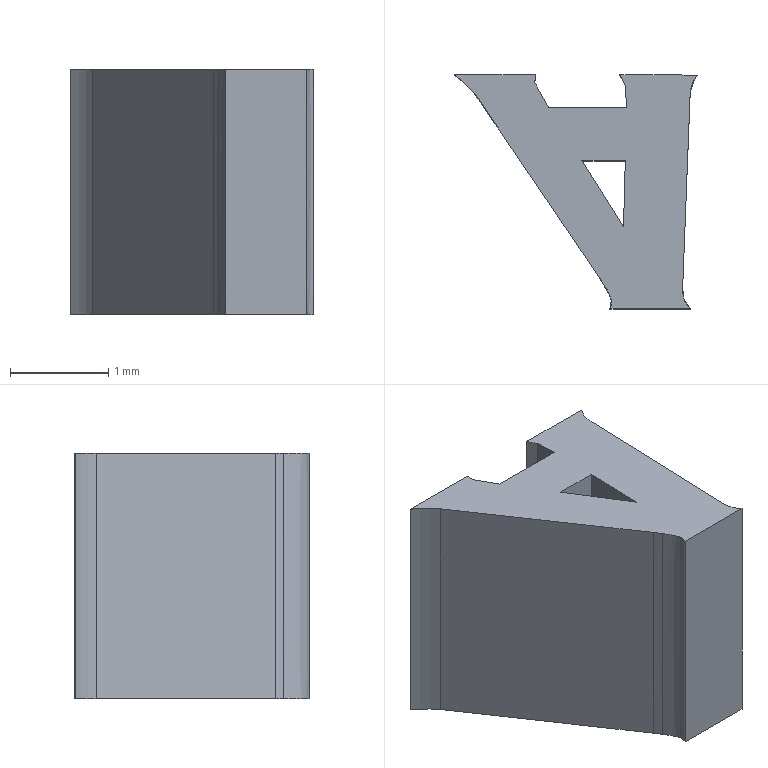Part | STEP file | lll_id1098_x_t | 1 solid | 20 faces | box 2.479 x 2.385 x 2.5 mm | volume 7.725 mm3 | plane 14 | other 4 | cylinder 2 | commonest cylinder face diameters 1.645 x1 55.723 x1
STEP:
#1=CARTESIAN_POINT('',(387.646,-127.04,2.35));
#2=VERTEX_POINT('',#1);
#3=CARTESIAN_POINT('',(387.664,-126.366,2.35));
#4=VERTEX_POINT('',#3);
#5=CARTESIAN_POINT('',(387.646,-127.04,2.35));
#6=DIRECTION('',(0.02693,0.9996,0.));
#7=VECTOR('',#6,1.);
#8=LINE('',#5,#7);
#9=EDGE_CURVE('',#2,#4,#8,.T.);
#10=ORIENTED_EDGE('',*,*,#9,.T.);
#11=CARTESIAN_POINT('',(387.664,-126.366,-0.15));
#12=VERTEX_POINT('',#11);
#13=CARTESIAN_POINT('',(387.664,-126.366,-0.15));
#14=DIRECTION('',(0.,0.,1.));
#15=VECTOR('',#14,1.);
#16=LINE('',#13,#15);
#17=EDGE_CURVE('',#12,#4,#16,.T.);
#18=ORIENTED_EDGE('',*,*,#17,.F.);
#19=CARTESIAN_POINT('',(387.646,-127.04,-0.15));
#20=VERTEX_POINT('',#19);
#21=CARTESIAN_POINT('',(387.646,-127.04,-0.15));
#22=DIRECTION('',(0.02693,0.9996,0.));
#23=VECTOR('',#22,1.);
#24=LINE('',#21,#23);
#25=EDGE_CURVE('',#20,#12,#24,.T.);
#26=ORIENTED_EDGE('',*,*,#25,.F.);
#27=CARTESIAN_POINT('',(387.646,-127.04,-0.15));
#28=DIRECTION('',(0.,0.,1.));
#29=VECTOR('',#28,1.);
#30=LINE('',#27,#29);
#31=EDGE_CURVE('',#20,#2,#30,.T.);
#32=ORIENTED_EDGE('',*,*,#31,.T.);
#33=EDGE_LOOP('',(#10,#18,#26,#32));
#34=FACE_OUTER_BOUND('',#33,.T.);
#35=CARTESIAN_POINT('',(387.646,-127.04,-0.15));
#36=DIRECTION('',(0.9996,-0.02693,0.));
#37=DIRECTION('',(-0.02693,-0.9996,0.));
#38=AXIS2_PLACEMENT_3D('',#35,#36,#37);
#39=PLANE('',#38);
#40=ADVANCED_FACE('',(#34),#39,.F.);
#41=CARTESIAN_POINT('',(387.223,-126.366,2.35));
#42=VERTEX_POINT('',#41);
#43=CARTESIAN_POINT('',(387.664,-126.366,2.35));
#44=DIRECTION('',(-1.,0.,0.));
#45=VECTOR('',#44,1.);
#46=LINE('',#43,#45);
#47=EDGE_CURVE('',#4,#42,#46,.T.);
#48=ORIENTED_EDGE('',*,*,#47,.T.);
#49=CARTESIAN_POINT('',(387.223,-126.366,-0.15));
#50=VERTEX_POINT('',#49);
#51=CARTESIAN_POINT('',(387.223,-126.366,-0.15));
#52=DIRECTION('',(0.,0.,1.));
#53=VECTOR('',#52,1.);
#54=LINE('',#51,#53);
#55=EDGE_CURVE('',#50,#42,#54,.T.);
#56=ORIENTED_EDGE('',*,*,#55,.F.);
#57=CARTESIAN_POINT('',(387.664,-126.366,-0.15));
#58=DIRECTION('',(-1.,0.,0.));
#59=VECTOR('',#58,1.);
#60=LINE('',#57,#59);
#61=EDGE_CURVE('',#12,#50,#60,.T.);
#62=ORIENTED_EDGE('',*,*,#61,.F.);
#63=ORIENTED_EDGE('',*,*,#17,.T.);
#64=EDGE_LOOP('',(#48,#56,#62,#63));
#65=FACE_OUTER_BOUND('',#64,.T.);
#66=CARTESIAN_POINT('',(387.664,-126.366,-0.15));
#67=DIRECTION('',(0.,1.,0.));
#68=DIRECTION('',(0.,0.,1.));
#69=AXIS2_PLACEMENT_3D('',#66,#67,#68);
#70=PLANE('',#69);
#71=ADVANCED_FACE('',(#65),#70,.F.);
#72=CARTESIAN_POINT('',(388.398,-125.498,2.35));
#73=VERTEX_POINT('',#72);
#74=CARTESIAN_POINT('',(388.323,-125.704,2.35));
#75=VERTEX_POINT('',#74);
#76=CARTESIAN_POINT('',(388.398,-125.498,2.35));
#77=CARTESIAN_POINT('',(388.389,-125.508,2.35));
#78=CARTESIAN_POINT('',(388.38,-125.519,2.35));
#79=CARTESIAN_POINT('',(388.363,-125.544,2.35));
#80=CARTESIAN_POINT('',(388.355,-125.559,2.35));
#81=CARTESIAN_POINT('',(388.343,-125.589,2.35));
#82=CARTESIAN_POINT('',(388.338,-125.605,2.35));
#83=CARTESIAN_POINT('',(388.331,-125.632,2.35));
#84=CARTESIAN_POINT('',(388.329,-125.644,2.35));
#85=CARTESIAN_POINT('',(388.325,-125.672,2.35));
#86=CARTESIAN_POINT('',(388.324,-125.688,2.35));
#87=CARTESIAN_POINT('',(388.323,-125.704,2.35));
#88=(BOUNDED_CURVE()B_SPLINE_CURVE(3,(#76,#77,#78,#79,#80,#81,#82,#83,#84,#85,#86,#87),.UNSPECIFIED.,.F.,.F.)B_SPLINE_CURVE_WITH_KNOTS((4,2,2,2,2,4),(0.,0.1892,0.4077,0.6263,0.7817,1.),.UNSPECIFIED.)CURVE()GEOMETRIC_REPRESENTATION_ITEM()RATIONAL_B_SPLINE_CURVE((0.5006,0.4998,0.4998,0.499,0.499,0.4995,0.4995,0.5003,0.5003,0.5002,0.5002,0.5006))REPRESENTATION_ITEM(''));
#89=EDGE_CURVE('',#73,#75,#88,.T.);
#90=ORIENTED_EDGE('',*,*,#89,.T.);
#91=CARTESIAN_POINT('',(388.323,-125.704,-0.15));
#92=VERTEX_POINT('',#91);
#93=CARTESIAN_POINT('',(388.323,-125.704,-0.15));
#94=DIRECTION('',(0.,0.,1.));
#95=VECTOR('',#94,1.);
#96=LINE('',#93,#95);
#97=EDGE_CURVE('',#92,#75,#96,.T.);
#98=ORIENTED_EDGE('',*,*,#97,.F.);
#99=CARTESIAN_POINT('',(388.398,-125.498,-0.15));
#100=VERTEX_POINT('',#99);
#101=CARTESIAN_POINT('',(388.398,-125.498,-0.15));
#102=CARTESIAN_POINT('',(388.389,-125.508,-0.15));
#103=CARTESIAN_POINT('',(388.38,-125.519,-0.15));
#104=CARTESIAN_POINT('',(388.363,-125.544,-0.15));
#105=CARTESIAN_POINT('',(388.355,-125.559,-0.15));
#106=CARTESIAN_POINT('',(388.343,-125.589,-0.15));
#107=CARTESIAN_POINT('',(388.338,-125.605,-0.15));
#108=CARTESIAN_POINT('',(388.331,-125.632,-0.15));
#109=CARTESIAN_POINT('',(388.329,-125.644,-0.15));
#110=CARTESIAN_POINT('',(388.325,-125.672,-0.15));
#111=CARTESIAN_POINT('',(388.324,-125.688,-0.15));
#112=CARTESIAN_POINT('',(388.323,-125.704,-0.15));
#113=(BOUNDED_CURVE()B_SPLINE_CURVE(3,(#101,#102,#103,#104,#105,#106,#107,#108,#109,#110,#111,#112),.UNSPECIFIED.,.F.,.F.)B_SPLINE_CURVE_WITH_KNOTS((4,2,2,2,2,4),(0.,0.1892,0.4077,0.6263,0.7817,1.),.UNSPECIFIED.)CURVE()GEOMETRIC_REPRESENTATION_ITEM()RATIONAL_B_SPLINE_CURVE((0.5006,0.4998,0.4998,0.499,0.499,0.4995,0.4995,0.5003,0.5003,0.5002,0.5002,0.5006))REPRESENTATION_ITEM(''));
#114=EDGE_CURVE('',#100,#92,#113,.T.);
#115=ORIENTED_EDGE('',*,*,#114,.F.);
#116=CARTESIAN_POINT('',(388.398,-125.498,-0.15));
#117=DIRECTION('',(0.,0.,1.));
#118=VECTOR('',#117,1.);
#119=LINE('',#116,#118);
#120=EDGE_CURVE('',#100,#73,#119,.T.);
#121=ORIENTED_EDGE('',*,*,#120,.T.);
#122=EDGE_LOOP('',(#90,#98,#115,#121));
#123=FACE_OUTER_BOUND('',#122,.T.);
#124=CARTESIAN_POINT('',(388.398,-125.498,-0.15));
#125=CARTESIAN_POINT('',(388.389,-125.508,-0.15));
#126=CARTESIAN_POINT('',(388.38,-125.519,-0.15));
#127=CARTESIAN_POINT('',(388.363,-125.544,-0.15));
#128=CARTESIAN_POINT('',(388.355,-125.559,-0.15));
#129=CARTESIAN_POINT('',(388.343,-125.589,-0.15));
#130=CARTESIAN_POINT('',(388.338,-125.605,-0.15));
#131=CARTESIAN_POINT('',(388.331,-125.632,-0.15));
#132=CARTESIAN_POINT('',(388.329,-125.644,-0.15));
#133=CARTESIAN_POINT('',(388.325,-125.672,-0.15));
#134=CARTESIAN_POINT('',(388.324,-125.688,-0.15));
#135=CARTESIAN_POINT('',(388.323,-125.704,-0.15));
#136=(BOUNDED_CURVE()B_SPLINE_CURVE(3,(#124,#125,#126,#127,#128,#129,#130,#131,#132,#133,#134,#135),.UNSPECIFIED.,.F.,.F.)B_SPLINE_CURVE_WITH_KNOTS((4,2,2,2,2,4),(0.,0.1892,0.4077,0.6263,0.7817,1.),.UNSPECIFIED.)CURVE()GEOMETRIC_REPRESENTATION_ITEM()RATIONAL_B_SPLINE_CURVE((0.5006,0.4998,0.4998,0.499,0.499,0.4995,0.4995,0.5003,0.5003,0.5002,0.5002,0.5006))REPRESENTATION_ITEM(''));
#137=DIRECTION('',(0.,0.,1.));
#138=VECTOR('',#137,1.);
#139=SURFACE_OF_LINEAR_EXTRUSION('',#136,#138);
#140=ADVANCED_FACE('',(#123),#139,.F.);
#141=CARTESIAN_POINT('',(388.247,-127.665,2.35));
#142=VERTEX_POINT('',#141);
#143=CARTESIAN_POINT('',(388.323,-125.704,2.35));
#144=DIRECTION('',(-0.0386,-0.9993,0.));
#145=VECTOR('',#144,1.);
#146=LINE('',#143,#145);
#147=EDGE_CURVE('',#75,#142,#146,.T.);
#148=ORIENTED_EDGE('',*,*,#147,.T.);
#149=CARTESIAN_POINT('',(388.247,-127.665,-0.15));
#150=VERTEX_POINT('',#149);
#151=CARTESIAN_POINT('',(388.247,-127.665,-0.15));
#152=DIRECTION('',(0.,0.,1.));
#153=VECTOR('',#152,1.);
#154=LINE('',#151,#153);
#155=EDGE_CURVE('',#150,#142,#154,.T.);
#156=ORIENTED_EDGE('',*,*,#155,.F.);
#157=CARTESIAN_POINT('',(388.323,-125.704,-0.15));
#158=DIRECTION('',(-0.0386,-0.9993,0.));
#159=VECTOR('',#158,1.);
#160=LINE('',#157,#159);
#161=EDGE_CURVE('',#92,#150,#160,.T.);
#162=ORIENTED_EDGE('',*,*,#161,.F.);
#163=ORIENTED_EDGE('',*,*,#97,.T.);
#164=EDGE_LOOP('',(#148,#156,#162,#163));
#165=FACE_OUTER_BOUND('',#164,.T.);
#166=CARTESIAN_POINT('',(388.323,-125.704,-0.15));
#167=DIRECTION('',(-0.9993,0.0386,0.));
#168=DIRECTION('',(0.0386,0.9993,0.));
#169=AXIS2_PLACEMENT_3D('',#166,#167,#168);
#170=PLANE('',#169);
#171=ADVANCED_FACE('',(#165),#170,.F.);
#172=CARTESIAN_POINT('',(388.323,-127.874,2.35));
#173=VERTEX_POINT('',#172);
#174=CARTESIAN_POINT('',(388.247,-127.665,2.35));
#175=CARTESIAN_POINT('',(388.246,-127.686,2.35));
#176=CARTESIAN_POINT('',(388.248,-127.708,2.35));
#177=CARTESIAN_POINT('',(388.253,-127.746,2.35));
#178=CARTESIAN_POINT('',(388.257,-127.762,2.35));
#179=CARTESIAN_POINT('',(388.271,-127.802,2.35));
#180=CARTESIAN_POINT('',(388.283,-127.825,2.35));
#181=CARTESIAN_POINT('',(388.307,-127.855,2.35));
#182=CARTESIAN_POINT('',(388.315,-127.864,2.35));
#183=CARTESIAN_POINT('',(388.324,-127.872,2.35));
#184=(BOUNDED_CURVE()B_SPLINE_CURVE(3,(#174,#175,#176,#177,#178,#179,#180,#181,#182,#183),.UNSPECIFIED.,.F.,.F.)B_SPLINE_CURVE_WITH_KNOTS((4,2,2,2,4),(0.,0.2836,0.5035,0.8455,1.),.UNSPECIFIED.)CURVE()GEOMETRIC_REPRESENTATION_ITEM()RATIONAL_B_SPLINE_CURVE((0.5011,0.4996,0.4996,0.4997,0.4997,0.4954,0.4954,0.5003,0.5003,0.5011))REPRESENTATION_ITEM(''));
#185=EDGE_CURVE('',#142,#173,#184,.T.);
#186=ORIENTED_EDGE('',*,*,#185,.T.);
#187=CARTESIAN_POINT('',(388.323,-127.874,-0.15));
#188=VERTEX_POINT('',#187);
#189=CARTESIAN_POINT('',(388.329,-127.876,-0.15));
#190=DIRECTION('',(0.,0.,1.));
#191=VECTOR('',#190,1.);
#192=LINE('',#189,#191);
#193=EDGE_CURVE('',#188,#173,#192,.T.);
#194=ORIENTED_EDGE('',*,*,#193,.F.);
#195=CARTESIAN_POINT('',(388.247,-127.665,-0.15));
#196=CARTESIAN_POINT('',(388.246,-127.686,-0.15));
#197=CARTESIAN_POINT('',(388.248,-127.708,-0.15));
#198=CARTESIAN_POINT('',(388.253,-127.746,-0.15));
#199=CARTESIAN_POINT('',(388.257,-127.762,-0.15));
#200=CARTESIAN_POINT('',(388.271,-127.802,-0.15));
#201=CARTESIAN_POINT('',(388.283,-127.825,-0.15));
#202=CARTESIAN_POINT('',(388.307,-127.855,-0.15));
#203=CARTESIAN_POINT('',(388.315,-127.864,-0.15));
#204=CARTESIAN_POINT('',(388.325,-127.872,-0.15));
#205=CARTESIAN_POINT('',(388.325,-127.873,-0.15));
#206=CARTESIAN_POINT('',(388.326,-127.873,-0.15));
#207=(BOUNDED_CURVE()B_SPLINE_CURVE(3,(#195,#196,#197,#198,#199,#200,#201,#202,#203,#204,#205,#206),.UNSPECIFIED.,.F.,.F.)B_SPLINE_CURVE_WITH_KNOTS((4,2,2,2,2,4),(0.,0.2808,0.4985,0.8371,0.9901,1.),.UNSPECIFIED.)CURVE()GEOMETRIC_REPRESENTATION_ITEM()RATIONAL_B_SPLINE_CURVE((0.5011,0.4996,0.4996,0.4997,0.4997,0.4954,0.4954,0.5003,0.5003,0.5011,0.5011,0.5011))REPRESENTATION_ITEM(''));
#208=EDGE_CURVE('',#150,#188,#207,.T.);
#209=ORIENTED_EDGE('',*,*,#208,.F.);
#210=ORIENTED_EDGE('',*,*,#155,.T.);
#211=EDGE_LOOP('',(#186,#194,#209,#210));
#212=FACE_OUTER_BOUND('',#211,.T.);
#213=CARTESIAN_POINT('',(388.247,-127.665,-0.15));
#214=CARTESIAN_POINT('',(388.246,-127.686,-0.15));
#215=CARTESIAN_POINT('',(388.248,-127.708,-0.15));
#216=CARTESIAN_POINT('',(388.253,-127.746,-0.15));
#217=CARTESIAN_POINT('',(388.257,-127.762,-0.15));
#218=CARTESIAN_POINT('',(388.271,-127.802,-0.15));
#219=CARTESIAN_POINT('',(388.283,-127.825,-0.15));
#220=CARTESIAN_POINT('',(388.307,-127.855,-0.15));
#221=CARTESIAN_POINT('',(388.315,-127.864,-0.15));
#222=CARTESIAN_POINT('',(388.325,-127.872,-0.15));
#223=CARTESIAN_POINT('',(388.325,-127.873,-0.15));
#224=CARTESIAN_POINT('',(388.326,-127.874,-0.15));
#225=CARTESIAN_POINT('',(388.327,-127.874,-0.15));
#226=CARTESIAN_POINT('',(388.328,-127.875,-0.15));
#227=CARTESIAN_POINT('',(388.328,-127.876,-0.15));
#228=CARTESIAN_POINT('',(388.329,-127.876,-0.15));
#229=(BOUNDED_CURVE()B_SPLINE_CURVE(3,(#213,#214,#215,#216,#217,#218,#219,#220,#221,#222,#223,#224,#225,#226,#227,#228),.UNSPECIFIED.,.F.,.F.)B_SPLINE_CURVE_WITH_KNOTS((4,2,2,2,2,2,2,4),(0.,0.2753,0.4887,0.8206,0.9706,0.9803,0.9901,1.),.UNSPECIFIED.)CURVE()GEOMETRIC_REPRESENTATION_ITEM()RATIONAL_B_SPLINE_CURVE((0.5011,0.4996,0.4996,0.4997,0.4997,0.4954,0.4954,0.5003,0.5003,0.5011,0.5011,0.5011,0.5011,0.5011,0.5011,0.5011))REPRESENTATION_ITEM(''));
#230=DIRECTION('',(0.,0.,1.));
#231=VECTOR('',#230,1.);
#232=SURFACE_OF_LINEAR_EXTRUSION('',#229,#231);
#233=ADVANCED_FACE('',(#212),#232,.F.);
#234=CARTESIAN_POINT('',(387.509,-127.874,2.35));
#235=VERTEX_POINT('',#234);
#236=CARTESIAN_POINT('',(388.323,-127.876,2.35));
#237=DIRECTION('',(-1.,0.,0.));
#238=VECTOR('',#237,1.);
#239=LINE('',#236,#238);
#240=EDGE_CURVE('',#173,#235,#239,.T.);
#241=ORIENTED_EDGE('',*,*,#240,.T.);
#242=CARTESIAN_POINT('',(387.509,-127.874,-0.15));
#243=VERTEX_POINT('',#242);
#244=CARTESIAN_POINT('',(387.507,-127.876,-0.15));
#245=DIRECTION('',(0.,0.,1.));
#246=VECTOR('',#245,1.);
#247=LINE('',#244,#246);
#248=EDGE_CURVE('',#243,#235,#247,.T.);
#249=ORIENTED_EDGE('',*,*,#248,.F.);
#250=CARTESIAN_POINT('',(388.323,-127.876,-0.15));
#251=DIRECTION('',(-1.,0.,0.));
#252=VECTOR('',#251,1.);
#253=LINE('',#250,#252);
#254=EDGE_CURVE('',#188,#243,#253,.T.);
#255=ORIENTED_EDGE('',*,*,#254,.F.);
#256=ORIENTED_EDGE('',*,*,#193,.T.);
#257=EDGE_LOOP('',(#241,#249,#255,#256));
#258=FACE_OUTER_BOUND('',#257,.T.);
#259=CARTESIAN_POINT('',(388.323,-127.876,-0.15));
#260=DIRECTION('',(0.,1.,0.));
#261=DIRECTION('',(0.,0.,1.));
#262=AXIS2_PLACEMENT_3D('',#259,#260,#261);
#263=PLANE('',#262);
#264=ADVANCED_FACE('',(#258),#263,.F.);
#265=CARTESIAN_POINT('',(387.437,-127.612,2.35));
#266=VERTEX_POINT('',#265);
#267=CARTESIAN_POINT('',(387.509,-127.872,2.35));
#268=CARTESIAN_POINT('',(387.511,-127.867,2.35));
#269=CARTESIAN_POINT('',(387.513,-127.861,2.35));
#270=CARTESIAN_POINT('',(387.523,-127.833,2.35));
#271=CARTESIAN_POINT('',(387.524,-127.809,2.35));
#272=CARTESIAN_POINT('',(387.518,-127.772,2.35));
#273=CARTESIAN_POINT('',(387.515,-127.759,2.35));
#274=CARTESIAN_POINT('',(387.507,-127.739,2.35));
#275=CARTESIAN_POINT('',(387.504,-127.731,2.35));
#276=CARTESIAN_POINT('',(387.496,-127.714,2.35));
#277=CARTESIAN_POINT('',(387.491,-127.703,2.35));
#278=CARTESIAN_POINT('',(387.48,-127.683,2.35));
#279=CARTESIAN_POINT('',(387.474,-127.672,2.35));
#280=CARTESIAN_POINT('',(387.458,-127.646,2.35));
#281=CARTESIAN_POINT('',(387.447,-127.629,2.35));
#282=CARTESIAN_POINT('',(387.437,-127.612,2.35));
#283=(BOUNDED_CURVE()B_SPLINE_CURVE(3,(#267,#268,#269,#270,#271,#272,#273,#274,#275,#276,#277,#278,#279,#280,#281,#282),.UNSPECIFIED.,.F.,.F.)B_SPLINE_CURVE_WITH_KNOTS((4,2,2,2,2,2,2,4),(0.,0.06399,0.3162,0.4617,0.5445,0.6686,0.7929,1.),.UNSPECIFIED.)CURVE()GEOMETRIC_REPRESENTATION_ITEM()RATIONAL_B_SPLINE_CURVE((0.5002,0.4999,0.4999,0.4907,0.4907,0.4986,0.4986,0.5,0.5,0.5,0.5,0.5002,0.5002,0.5002,0.5002,0.5002))REPRESENTATION_ITEM(''));
#284=EDGE_CURVE('',#235,#266,#283,.T.);
#285=ORIENTED_EDGE('',*,*,#284,.T.);
#286=CARTESIAN_POINT('',(387.437,-127.612,-0.15));
#287=VERTEX_POINT('',#286);
#288=CARTESIAN_POINT('',(387.437,-127.612,-0.15));
#289=DIRECTION('',(0.,0.,1.));
#290=VECTOR('',#289,1.);
#291=LINE('',#288,#290);
#292=EDGE_CURVE('',#287,#266,#291,.T.);
#293=ORIENTED_EDGE('',*,*,#292,.F.);
#294=CARTESIAN_POINT('',(387.507,-127.874,-0.15));
#295=CARTESIAN_POINT('',(387.508,-127.874,-0.15));
#296=CARTESIAN_POINT('',(387.508,-127.873,-0.15));
#297=CARTESIAN_POINT('',(387.511,-127.867,-0.15));
#298=CARTESIAN_POINT('',(387.513,-127.861,-0.15));
#299=CARTESIAN_POINT('',(387.523,-127.833,-0.15));
#300=CARTESIAN_POINT('',(387.524,-127.809,-0.15));
#301=CARTESIAN_POINT('',(387.518,-127.772,-0.15));
#302=CARTESIAN_POINT('',(387.515,-127.759,-0.15));
#303=CARTESIAN_POINT('',(387.507,-127.739,-0.15));
#304=CARTESIAN_POINT('',(387.504,-127.731,-0.15));
#305=CARTESIAN_POINT('',(387.496,-127.714,-0.15));
#306=CARTESIAN_POINT('',(387.491,-127.703,-0.15));
#307=CARTESIAN_POINT('',(387.48,-127.683,-0.15));
#308=CARTESIAN_POINT('',(387.474,-127.672,-0.15));
#309=CARTESIAN_POINT('',(387.458,-127.646,-0.15));
#310=CARTESIAN_POINT('',(387.447,-127.629,-0.15));
#311=CARTESIAN_POINT('',(387.437,-127.612,-0.15));
#312=(BOUNDED_CURVE()B_SPLINE_CURVE(3,(#294,#295,#296,#297,#298,#299,#300,#301,#302,#303,#304,#305,#306,#307,#308,#309,#310,#311),.UNSPECIFIED.,.F.,.F.)B_SPLINE_CURVE_WITH_KNOTS((4,2,2,2,2,2,2,2,4),(0.,0.009901,0.07326,0.323,0.467,0.549,0.6718,0.795,1.),.UNSPECIFIED.)CURVE()GEOMETRIC_REPRESENTATION_ITEM()RATIONAL_B_SPLINE_CURVE((0.5002,0.5002,0.5002,0.4999,0.4999,0.4907,0.4907,0.4986,0.4986,0.5,0.5,0.5,0.5,0.5002,0.5002,0.5002,0.5002,0.5002))REPRESENTATION_ITEM(''));
#313=EDGE_CURVE('',#243,#287,#312,.T.);
#314=ORIENTED_EDGE('',*,*,#313,.F.);
#315=ORIENTED_EDGE('',*,*,#248,.T.);
#316=EDGE_LOOP('',(#285,#293,#314,#315));
#317=FACE_OUTER_BOUND('',#316,.T.);
#318=CARTESIAN_POINT('',(387.506,-127.877,-0.15));
#319=CARTESIAN_POINT('',(387.507,-127.876,-0.15));
#320=CARTESIAN_POINT('',(387.507,-127.875,-0.15));
#321=CARTESIAN_POINT('',(387.508,-127.874,-0.15));
#322=CARTESIAN_POINT('',(387.508,-127.873,-0.15));
#323=CARTESIAN_POINT('',(387.511,-127.867,-0.15));
#324=CARTESIAN_POINT('',(387.513,-127.861,-0.15));
#325=CARTESIAN_POINT('',(387.523,-127.833,-0.15));
#326=CARTESIAN_POINT('',(387.524,-127.809,-0.15));
#327=CARTESIAN_POINT('',(387.518,-127.772,-0.15));
#328=CARTESIAN_POINT('',(387.515,-127.759,-0.15));
#329=CARTESIAN_POINT('',(387.507,-127.739,-0.15));
#330=CARTESIAN_POINT('',(387.504,-127.731,-0.15));
#331=CARTESIAN_POINT('',(387.496,-127.714,-0.15));
#332=CARTESIAN_POINT('',(387.491,-127.703,-0.15));
#333=CARTESIAN_POINT('',(387.48,-127.683,-0.15));
#334=CARTESIAN_POINT('',(387.474,-127.672,-0.15));
#335=CARTESIAN_POINT('',(387.458,-127.646,-0.15));
#336=CARTESIAN_POINT('',(387.447,-127.629,-0.15));
#337=CARTESIAN_POINT('',(387.437,-127.612,-0.15));
#338=(BOUNDED_CURVE()B_SPLINE_CURVE(3,(#318,#319,#320,#321,#322,#323,#324,#325,#326,#327,#328,#329,#330,#331,#332,#333,#334,#335,#336,#337),.UNSPECIFIED.,.F.,.F.)B_SPLINE_CURVE_WITH_KNOTS((4,2,2,2,2,2,2,2,2,4),(0.,0.009901,0.0197,0.08244,0.3297,0.4723,0.5535,0.6751,0.797,1.),.UNSPECIFIED.)CURVE()GEOMETRIC_REPRESENTATION_ITEM()RATIONAL_B_SPLINE_CURVE((0.5002,0.5002,0.5002,0.5002,0.5002,0.4999,0.4999,0.4907,0.4907,0.4986,0.4986,0.5,0.5,0.5,0.5,0.5002,0.5002,0.5002,0.5002,0.5002))REPRESENTATION_ITEM(''));
#339=DIRECTION('',(0.,0.,1.));
#340=VECTOR('',#339,1.);
#341=SURFACE_OF_LINEAR_EXTRUSION('',#338,#340);
#342=ADVANCED_FACE('',(#317),#341,.F.);
#343=CARTESIAN_POINT('',(387.387,-127.533,2.35));
#344=VERTEX_POINT('',#343);
#345=CARTESIAN_POINT('',(387.437,-127.612,2.35));
#346=CARTESIAN_POINT('',(387.429,-127.599,2.35));
#347=CARTESIAN_POINT('',(387.421,-127.585,2.35));
#348=CARTESIAN_POINT('',(387.404,-127.559,2.35));
#349=CARTESIAN_POINT('',(387.396,-127.546,2.35));
#350=CARTESIAN_POINT('',(387.387,-127.533,2.35));
#351=(BOUNDED_CURVE()B_SPLINE_CURVE(3,(#345,#346,#347,#348,#349,#350),.UNSPECIFIED.,.F.,.F.)B_SPLINE_CURVE_WITH_KNOTS((4,2,4),(0.,0.5001,1.),.UNSPECIFIED.)CURVE()GEOMETRIC_REPRESENTATION_ITEM()RATIONAL_B_SPLINE_CURVE((0.5002,0.5002,0.5002,0.5002,0.5002,0.5002))REPRESENTATION_ITEM(''));
#352=EDGE_CURVE('',#266,#344,#351,.T.);
#353=ORIENTED_EDGE('',*,*,#352,.T.);
#354=CARTESIAN_POINT('',(387.387,-127.533,-0.15));
#355=VERTEX_POINT('',#354);
#356=CARTESIAN_POINT('',(387.387,-127.533,-0.15));
#357=DIRECTION('',(0.,0.,1.));
#358=VECTOR('',#357,1.);
#359=LINE('',#356,#358);
#360=EDGE_CURVE('',#355,#344,#359,.T.);
#361=ORIENTED_EDGE('',*,*,#360,.F.);
#362=CARTESIAN_POINT('',(387.437,-127.612,-0.15));
#363=CARTESIAN_POINT('',(387.429,-127.599,-0.15));
#364=CARTESIAN_POINT('',(387.421,-127.585,-0.15));
#365=CARTESIAN_POINT('',(387.404,-127.559,-0.15));
#366=CARTESIAN_POINT('',(387.396,-127.546,-0.15));
#367=CARTESIAN_POINT('',(387.387,-127.533,-0.15));
#368=(BOUNDED_CURVE()B_SPLINE_CURVE(3,(#362,#363,#364,#365,#366,#367),.UNSPECIFIED.,.F.,.F.)B_SPLINE_CURVE_WITH_KNOTS((4,2,4),(0.,0.5001,1.),.UNSPECIFIED.)CURVE()GEOMETRIC_REPRESENTATION_ITEM()RATIONAL_B_SPLINE_CURVE((0.5002,0.5002,0.5002,0.5002,0.5002,0.5002))REPRESENTATION_ITEM(''));
#369=EDGE_CURVE('',#287,#355,#368,.T.);
#370=ORIENTED_EDGE('',*,*,#369,.F.);
#371=ORIENTED_EDGE('',*,*,#292,.T.);
#372=EDGE_LOOP('',(#353,#361,#370,#371));
#373=FACE_OUTER_BOUND('',#372,.T.);
#374=CARTESIAN_POINT('',(387.437,-127.612,-0.15));
#375=CARTESIAN_POINT('',(387.429,-127.599,-0.15));
#376=CARTESIAN_POINT('',(387.421,-127.585,-0.15));
#377=CARTESIAN_POINT('',(387.404,-127.559,-0.15));
#378=CARTESIAN_POINT('',(387.396,-127.546,-0.15));
#379=CARTESIAN_POINT('',(387.387,-127.533,-0.15));
#380=(BOUNDED_CURVE()B_SPLINE_CURVE(3,(#374,#375,#376,#377,#378,#379),.UNSPECIFIED.,.F.,.F.)B_SPLINE_CURVE_WITH_KNOTS((4,2,4),(0.,0.5001,1.),.UNSPECIFIED.)CURVE()GEOMETRIC_REPRESENTATION_ITEM()RATIONAL_B_SPLINE_CURVE((0.5002,0.5002,0.5002,0.5002,0.5002,0.5002))REPRESENTATION_ITEM(''));
#381=DIRECTION('',(0.,0.,1.));
#382=VECTOR('',#381,1.);
#383=SURFACE_OF_LINEAR_EXTRUSION('',#380,#382);
#384=ADVANCED_FACE('',(#373),#383,.F.);
#385=CARTESIAN_POINT('',(386.149,-125.708,2.35));
#386=VERTEX_POINT('',#385);
#387=CARTESIAN_POINT('',(387.387,-127.533,2.35));
#388=DIRECTION('',(-0.5613,0.8276,0.));
#389=VECTOR('',#388,1.);
#390=LINE('',#387,#389);
#391=EDGE_CURVE('',#344,#386,#390,.T.);
#392=ORIENTED_EDGE('',*,*,#391,.T.);
#393=CARTESIAN_POINT('',(386.149,-125.708,-0.15));
#394=VERTEX_POINT('',#393);
#395=CARTESIAN_POINT('',(386.149,-125.708,-0.15));
#396=DIRECTION('',(0.,0.,1.));
#397=VECTOR('',#396,1.);
#398=LINE('',#395,#397);
#399=EDGE_CURVE('',#394,#386,#398,.T.);
#400=ORIENTED_EDGE('',*,*,#399,.F.);
#401=CARTESIAN_POINT('',(387.387,-127.533,-0.15));
#402=DIRECTION('',(-0.5613,0.8276,0.));
#403=VECTOR('',#402,1.);
#404=LINE('',#401,#403);
#405=EDGE_CURVE('',#355,#394,#404,.T.);
#406=ORIENTED_EDGE('',*,*,#405,.F.);
#407=ORIENTED_EDGE('',*,*,#360,.T.);
#408=EDGE_LOOP('',(#392,#400,#406,#407));
#409=FACE_OUTER_BOUND('',#408,.T.);
#410=CARTESIAN_POINT('',(387.387,-127.533,-0.15));
#411=DIRECTION('',(0.8276,0.5613,0.));
#412=DIRECTION('',(0.5613,-0.8276,0.));
#413=AXIS2_PLACEMENT_3D('',#410,#411,#412);
#414=PLANE('',#413);
#415=ADVANCED_FACE('',(#409),#414,.F.);
#416=CARTESIAN_POINT('',(385.928,-125.495,2.35));
#417=VERTEX_POINT('',#416);
#418=CARTESIAN_POINT('',(385.482,-126.189,2.35));
#419=DIRECTION('',(0.,0.,1.));
#420=DIRECTION('',(-1.,0.,0.));
#421=AXIS2_PLACEMENT_3D('',#418,#419,#420);
#422=CIRCLE('',#421,0.8223);
#423=EDGE_CURVE('',#386,#417,#422,.T.);
#424=ORIENTED_EDGE('',*,*,#423,.T.);
#425=CARTESIAN_POINT('',(385.928,-125.495,-0.15));
#426=VERTEX_POINT('',#425);
#427=CARTESIAN_POINT('',(385.919,-125.492,-0.15));
#428=DIRECTION('',(0.,0.,1.));
#429=VECTOR('',#428,1.);
#430=LINE('',#427,#429);
#431=EDGE_CURVE('',#426,#417,#430,.T.);
#432=ORIENTED_EDGE('',*,*,#431,.F.);
#433=CARTESIAN_POINT('',(385.482,-126.189,-0.15));
#434=DIRECTION('',(0.,0.,1.));
#435=DIRECTION('',(-1.,0.,0.));
#436=AXIS2_PLACEMENT_3D('',#433,#434,#435);
#437=CIRCLE('',#436,0.8223);
#438=EDGE_CURVE('',#394,#426,#437,.T.);
#439=ORIENTED_EDGE('',*,*,#438,.F.);
#440=ORIENTED_EDGE('',*,*,#399,.T.);
#441=EDGE_LOOP('',(#424,#432,#439,#440));
#442=FACE_OUTER_BOUND('',#441,.T.);
#443=CARTESIAN_POINT('',(385.482,-126.189,-0.15));
#444=DIRECTION('',(0.,0.,1.));
#445=DIRECTION('',(1.,0.,0.));
#446=AXIS2_PLACEMENT_3D('',#443,#444,#445);
#447=CYLINDRICAL_SURFACE('',#446,0.8223);
#448=ADVANCED_FACE('',(#442),#447,.F.);
#449=CARTESIAN_POINT('',(386.749,-125.494,2.35));
#450=VERTEX_POINT('',#449);
#451=CARTESIAN_POINT('',(385.928,-125.492,2.35));
#452=DIRECTION('',(1.,0.,0.));
#453=VECTOR('',#452,1.);
#454=LINE('',#451,#453);
#455=EDGE_CURVE('',#417,#450,#454,.T.);
#456=ORIENTED_EDGE('',*,*,#455,.T.);
#457=CARTESIAN_POINT('',(386.749,-125.494,-0.15));
#458=VERTEX_POINT('',#457);
#459=CARTESIAN_POINT('',(386.75,-125.492,-0.15));
#460=DIRECTION('',(0.,0.,1.));
#461=VECTOR('',#460,1.);
#462=LINE('',#459,#461);
#463=EDGE_CURVE('',#458,#450,#462,.T.);
#464=ORIENTED_EDGE('',*,*,#463,.F.);
#465=CARTESIAN_POINT('',(385.928,-125.492,-0.15));
#466=DIRECTION('',(1.,0.,0.));
#467=VECTOR('',#466,1.);
#468=LINE('',#465,#467);
#469=EDGE_CURVE('',#426,#458,#468,.T.);
#470=ORIENTED_EDGE('',*,*,#469,.F.);
#471=ORIENTED_EDGE('',*,*,#431,.T.);
#472=EDGE_LOOP('',(#456,#464,#470,#471));
#473=FACE_OUTER_BOUND('',#472,.T.);
#474=CARTESIAN_POINT('',(385.928,-125.492,-0.15));
#475=DIRECTION('',(0.,-1.,0.));
#476=DIRECTION('',(0.,0.,-1.));
#477=AXIS2_PLACEMENT_3D('',#474,#475,#476);
#478=PLANE('',#477);
#479=ADVANCED_FACE('',(#473),#478,.F.);
#480=CARTESIAN_POINT('',(386.745,-125.576,2.35));
#481=VERTEX_POINT('',#480);
#482=CARTESIAN_POINT('',(386.749,-125.496,2.35));
#483=DIRECTION('',(-0.05956,-0.9982,0.));
#484=VECTOR('',#483,1.);
#485=LINE('',#482,#484);
#486=EDGE_CURVE('',#450,#481,#485,.T.);
#487=ORIENTED_EDGE('',*,*,#486,.T.);
#488=CARTESIAN_POINT('',(386.745,-125.576,-0.15));
#489=VERTEX_POINT('',#488);
#490=CARTESIAN_POINT('',(386.745,-125.576,-0.15));
#491=DIRECTION('',(0.,0.,1.));
#492=VECTOR('',#491,1.);
#493=LINE('',#490,#492);
#494=EDGE_CURVE('',#489,#481,#493,.T.);
#495=ORIENTED_EDGE('',*,*,#494,.F.);
#496=CARTESIAN_POINT('',(386.749,-125.496,-0.15));
#497=DIRECTION('',(-0.05956,-0.9982,0.));
#498=VECTOR('',#497,1.);
#499=LINE('',#496,#498);
#500=EDGE_CURVE('',#458,#489,#499,.T.);
#501=ORIENTED_EDGE('',*,*,#500,.F.);
#502=ORIENTED_EDGE('',*,*,#463,.T.);
#503=EDGE_LOOP('',(#487,#495,#501,#502));
#504=FACE_OUTER_BOUND('',#503,.T.);
#505=CARTESIAN_POINT('',(386.749,-125.496,-0.15));
#506=DIRECTION('',(-0.9982,0.05956,0.));
#507=DIRECTION('',(0.05956,0.9982,0.));
#508=AXIS2_PLACEMENT_3D('',#505,#506,#507);
#509=PLANE('',#508);
#510=ADVANCED_FACE('',(#504),#509,.F.);
#511=CARTESIAN_POINT('',(386.885,-125.828,2.35));
#512=VERTEX_POINT('',#511);
#513=CARTESIAN_POINT('',(386.745,-125.576,2.35));
#514=DIRECTION('',(0.4861,-0.8739,0.));
#515=VECTOR('',#514,1.);
#516=LINE('',#513,#515);
#517=EDGE_CURVE('',#481,#512,#516,.T.);
#518=ORIENTED_EDGE('',*,*,#517,.T.);
#519=CARTESIAN_POINT('',(386.885,-125.828,-0.15));
#520=VERTEX_POINT('',#519);
#521=CARTESIAN_POINT('',(386.885,-125.828,-0.15));
#522=DIRECTION('',(0.,0.,1.));
#523=VECTOR('',#522,1.);
#524=LINE('',#521,#523);
#525=EDGE_CURVE('',#520,#512,#524,.T.);
#526=ORIENTED_EDGE('',*,*,#525,.F.);
#527=CARTESIAN_POINT('',(386.745,-125.576,-0.15));
#528=DIRECTION('',(0.4861,-0.8739,0.));
#529=VECTOR('',#528,1.);
#530=LINE('',#527,#529);
#531=EDGE_CURVE('',#489,#520,#530,.T.);
#532=ORIENTED_EDGE('',*,*,#531,.F.);
#533=ORIENTED_EDGE('',*,*,#494,.T.);
#534=EDGE_LOOP('',(#518,#526,#532,#533));
#535=FACE_OUTER_BOUND('',#534,.T.);
#536=CARTESIAN_POINT('',(386.745,-125.576,-0.15));
#537=DIRECTION('',(-0.8739,-0.4861,0.));
#538=DIRECTION('',(-0.4861,0.8739,0.));
#539=AXIS2_PLACEMENT_3D('',#536,#537,#538);
#540=PLANE('',#539);
#541=ADVANCED_FACE('',(#535),#540,.F.);
#542=CARTESIAN_POINT('',(387.679,-125.828,2.35));
#543=VERTEX_POINT('',#542);
#544=CARTESIAN_POINT('',(386.885,-125.828,2.35));
#545=DIRECTION('',(1.,0.,0.));
#546=VECTOR('',#545,1.);
#547=LINE('',#544,#546);
#548=EDGE_CURVE('',#512,#543,#547,.T.);
#549=ORIENTED_EDGE('',*,*,#548,.T.);
#550=CARTESIAN_POINT('',(387.679,-125.828,-0.15));
#551=VERTEX_POINT('',#550);
#552=CARTESIAN_POINT('',(387.679,-125.828,-0.15));
#553=DIRECTION('',(0.,0.,1.));
#554=VECTOR('',#553,1.);
#555=LINE('',#552,#554);
#556=EDGE_CURVE('',#551,#543,#555,.T.);
#557=ORIENTED_EDGE('',*,*,#556,.F.);
#558=CARTESIAN_POINT('',(386.885,-125.828,-0.15));
#559=DIRECTION('',(1.,0.,0.));
#560=VECTOR('',#559,1.);
#561=LINE('',#558,#560);
#562=EDGE_CURVE('',#520,#551,#561,.T.);
#563=ORIENTED_EDGE('',*,*,#562,.F.);
#564=ORIENTED_EDGE('',*,*,#525,.T.);
#565=EDGE_LOOP('',(#549,#557,#563,#564));
#566=FACE_OUTER_BOUND('',#565,.T.);
#567=CARTESIAN_POINT('',(386.885,-125.828,-0.15));
#568=DIRECTION('',(0.,-1.,0.));
#569=DIRECTION('',(0.,0.,-1.));
#570=AXIS2_PLACEMENT_3D('',#567,#568,#569);
#571=PLANE('',#570);
#572=ADVANCED_FACE('',(#566),#571,.F.);
#573=CARTESIAN_POINT('',(387.661,-125.59,2.35));
#574=VERTEX_POINT('',#573);
#575=CARTESIAN_POINT('',(387.679,-125.828,2.35));
#576=DIRECTION('',(-0.0742,0.9972,0.));
#577=VECTOR('',#576,1.);
#578=LINE('',#575,#577);
#579=EDGE_CURVE('',#543,#574,#578,.T.);
#580=ORIENTED_EDGE('',*,*,#579,.T.);
#581=CARTESIAN_POINT('',(387.661,-125.59,-0.15));
#582=VERTEX_POINT('',#581);
#583=CARTESIAN_POINT('',(387.661,-125.59,-0.15));
#584=DIRECTION('',(0.,0.,1.));
#585=VECTOR('',#584,1.);
#586=LINE('',#583,#585);
#587=EDGE_CURVE('',#582,#574,#586,.T.);
#588=ORIENTED_EDGE('',*,*,#587,.F.);
#589=CARTESIAN_POINT('',(387.679,-125.828,-0.15));
#590=DIRECTION('',(-0.0742,0.9972,0.));
#591=VECTOR('',#590,1.);
#592=LINE('',#589,#591);
#593=EDGE_CURVE('',#551,#582,#592,.T.);
#594=ORIENTED_EDGE('',*,*,#593,.F.);
#595=ORIENTED_EDGE('',*,*,#556,.T.);
#596=EDGE_LOOP('',(#580,#588,#594,#595));
#597=FACE_OUTER_BOUND('',#596,.T.);
#598=CARTESIAN_POINT('',(387.679,-125.828,-0.15));
#599=DIRECTION('',(0.9972,0.0742,0.));
#600=DIRECTION('',(0.0742,-0.9972,0.));
#601=AXIS2_PLACEMENT_3D('',#598,#599,#600);
#602=PLANE('',#601);
#603=ADVANCED_FACE('',(#597),#602,.F.);
#604=CARTESIAN_POINT('',(387.609,-125.492,2.35));
#605=VERTEX_POINT('',#604);
#606=CARTESIAN_POINT('',(387.661,-125.59,2.35));
#607=DIRECTION('',(-0.4706,0.8824,0.));
#608=VECTOR('',#607,1.);
#609=LINE('',#606,#608);
#610=EDGE_CURVE('',#574,#605,#609,.T.);
#611=ORIENTED_EDGE('',*,*,#610,.T.);
#612=CARTESIAN_POINT('',(387.609,-125.492,-0.15));
#613=VERTEX_POINT('',#612);
#614=CARTESIAN_POINT('',(387.609,-125.492,-0.15));
#615=DIRECTION('',(0.,0.,1.));
#616=VECTOR('',#615,1.);
#617=LINE('',#614,#616);
#618=EDGE_CURVE('',#613,#605,#617,.T.);
#619=ORIENTED_EDGE('',*,*,#618,.F.);
#620=CARTESIAN_POINT('',(387.661,-125.59,-0.15));
#621=DIRECTION('',(-0.4706,0.8824,0.));
#622=VECTOR('',#621,1.);
#623=LINE('',#620,#622);
#624=EDGE_CURVE('',#582,#613,#623,.T.);
#625=ORIENTED_EDGE('',*,*,#624,.F.);
#626=ORIENTED_EDGE('',*,*,#587,.T.);
#627=EDGE_LOOP('',(#611,#619,#625,#626));
#628=FACE_OUTER_BOUND('',#627,.T.);
#629=CARTESIAN_POINT('',(387.661,-125.59,-0.15));
#630=DIRECTION('',(0.8824,0.4706,0.));
#631=DIRECTION('',(0.4706,-0.8824,0.));
#632=AXIS2_PLACEMENT_3D('',#629,#630,#631);
#633=PLANE('',#632);
#634=ADVANCED_FACE('',(#628),#633,.F.);
#635=CARTESIAN_POINT('',(387.816,-153.353,2.35));
#636=DIRECTION('',(0.,0.,-1.));
#637=DIRECTION('',(-1.,0.,0.));
#638=AXIS2_PLACEMENT_3D('',#635,#636,#637);
#639=CIRCLE('',#638,27.862);
#640=EDGE_CURVE('',#605,#73,#639,.T.);
#641=ORIENTED_EDGE('',*,*,#640,.T.);
#642=ORIENTED_EDGE('',*,*,#120,.F.);
#643=CARTESIAN_POINT('',(387.816,-153.353,-0.15));
#644=DIRECTION('',(0.,0.,-1.));
#645=DIRECTION('',(-1.,0.,0.));
#646=AXIS2_PLACEMENT_3D('',#643,#644,#645);
#647=CIRCLE('',#646,27.862);
#648=EDGE_CURVE('',#613,#100,#647,.T.);
#649=ORIENTED_EDGE('',*,*,#648,.F.);
#650=ORIENTED_EDGE('',*,*,#618,.T.);
#651=EDGE_LOOP('',(#641,#642,#649,#650));
#652=FACE_OUTER_BOUND('',#651,.T.);
#653=CARTESIAN_POINT('',(387.816,-153.353,-0.15));
#654=DIRECTION('',(0.,0.,1.));
#655=DIRECTION('',(1.,0.,0.));
#656=AXIS2_PLACEMENT_3D('',#653,#654,#655);
#657=CYLINDRICAL_SURFACE('',#656,27.862);
#658=ADVANCED_FACE('',(#652),#657,.T.);
#659=CARTESIAN_POINT('',(387.223,-126.366,2.35));
#660=DIRECTION('',(0.5317,-0.8469,0.));
#661=VECTOR('',#660,1.);
#662=LINE('',#659,#661);
#663=EDGE_CURVE('',#42,#2,#662,.T.);
#664=ORIENTED_EDGE('',*,*,#663,.T.);
#665=ORIENTED_EDGE('',*,*,#31,.F.);
#666=CARTESIAN_POINT('',(387.223,-126.366,-0.15));
#667=DIRECTION('',(0.5317,-0.8469,0.));
#668=VECTOR('',#667,1.);
#669=LINE('',#666,#668);
#670=EDGE_CURVE('',#50,#20,#669,.T.);
#671=ORIENTED_EDGE('',*,*,#670,.F.);
#672=ORIENTED_EDGE('',*,*,#55,.T.);
#673=EDGE_LOOP('',(#664,#665,#671,#672));
#674=FACE_OUTER_BOUND('',#673,.T.);
#675=CARTESIAN_POINT('',(387.223,-126.366,-0.15));
#676=DIRECTION('',(-0.8469,-0.5317,0.));
#677=DIRECTION('',(-0.5317,0.8469,0.));
#678=AXIS2_PLACEMENT_3D('',#675,#676,#677);
#679=PLANE('',#678);
#680=ADVANCED_FACE('',(#674),#679,.F.);
#681=ORIENTED_EDGE('',*,*,#114,.T.);
#682=ORIENTED_EDGE('',*,*,#161,.T.);
#683=ORIENTED_EDGE('',*,*,#208,.T.);
#684=ORIENTED_EDGE('',*,*,#254,.T.);
#685=ORIENTED_EDGE('',*,*,#313,.T.);
#686=ORIENTED_EDGE('',*,*,#369,.T.);
#687=ORIENTED_EDGE('',*,*,#405,.T.);
#688=ORIENTED_EDGE('',*,*,#438,.T.);
#689=ORIENTED_EDGE('',*,*,#469,.T.);
#690=ORIENTED_EDGE('',*,*,#500,.T.);
#691=ORIENTED_EDGE('',*,*,#531,.T.);
#692=ORIENTED_EDGE('',*,*,#562,.T.);
#693=ORIENTED_EDGE('',*,*,#593,.T.);
#694=ORIENTED_EDGE('',*,*,#624,.T.);
#695=ORIENTED_EDGE('',*,*,#648,.T.);
#696=EDGE_LOOP('',(#681,#682,#683,#684,#685,#686,#687,#688,#689,#690,#691,#692,#693,#694,#695));
#697=FACE_BOUND('',#696,.T.);
#698=ORIENTED_EDGE('',*,*,#25,.T.);
#699=ORIENTED_EDGE('',*,*,#61,.T.);
#700=ORIENTED_EDGE('',*,*,#670,.T.);
#701=EDGE_LOOP('',(#698,#699,#700));
#702=FACE_BOUND('',#701,.T.);
#703=CARTESIAN_POINT('',(388.342,-125.594,-0.15));
#704=DIRECTION('',(0.,0.,-1.));
#705=DIRECTION('',(-1.,0.,0.));
#706=AXIS2_PLACEMENT_3D('',#703,#704,#705);
#707=PLANE('',#706);
#708=ADVANCED_FACE('',(#697,#702),#707,.T.);
#709=ORIENTED_EDGE('',*,*,#89,.F.);
#710=ORIENTED_EDGE('',*,*,#640,.F.);
#711=ORIENTED_EDGE('',*,*,#610,.F.);
#712=ORIENTED_EDGE('',*,*,#579,.F.);
#713=ORIENTED_EDGE('',*,*,#548,.F.);
#714=ORIENTED_EDGE('',*,*,#517,.F.);
#715=ORIENTED_EDGE('',*,*,#486,.F.);
#716=ORIENTED_EDGE('',*,*,#455,.F.);
#717=ORIENTED_EDGE('',*,*,#423,.F.);
#718=ORIENTED_EDGE('',*,*,#391,.F.);
#719=ORIENTED_EDGE('',*,*,#352,.F.);
#720=ORIENTED_EDGE('',*,*,#284,.F.);
#721=ORIENTED_EDGE('',*,*,#240,.F.);
#722=ORIENTED_EDGE('',*,*,#185,.F.);
#723=ORIENTED_EDGE('',*,*,#147,.F.);
#724=EDGE_LOOP('',(#709,#710,#711,#712,#713,#714,#715,#716,#717,#718,#719,#720,#721,#722,#723));
#725=FACE_BOUND('',#724,.T.);
#726=ORIENTED_EDGE('',*,*,#9,.F.);
#727=ORIENTED_EDGE('',*,*,#663,.F.);
#728=ORIENTED_EDGE('',*,*,#47,.F.);
#729=EDGE_LOOP('',(#726,#727,#728));
#730=FACE_BOUND('',#729,.T.);
#731=CARTESIAN_POINT('',(388.342,-125.594,2.35));
#732=DIRECTION('',(0.,0.,-1.));
#733=DIRECTION('',(-1.,0.,0.));
#734=AXIS2_PLACEMENT_3D('',#731,#732,#733);
#735=PLANE('',#734);
#736=ADVANCED_FACE('',(#725,#730),#735,.F.);
#737=CLOSED_SHELL('',(#40,#71,#140,#171,#233,#264,#342,#384,#415,#448,#479,#510,#541,#572,#603,#634,#658,#680,#708,#736));
#738=MANIFOLD_SOLID_BREP('',#737);
#739=(LENGTH_UNIT()NAMED_UNIT(*)SI_UNIT(.MILLI.,.METRE.));
#740=UNCERTAINTY_MEASURE_WITH_UNIT(LENGTH_MEASURE(0.01766),#739,'','');
#741=(NAMED_UNIT(*)PLANE_ANGLE_UNIT()SI_UNIT($,.RADIAN.));
#742=PLANE_ANGLE_MEASURE_WITH_UNIT(PLANE_ANGLE_MEASURE(0.01745),#741);
#743=DIMENSIONAL_EXPONENTS(0.,0.,0.,0.,0.,0.,0.);
#744=(CONVERSION_BASED_UNIT('DEGREE',#742)NAMED_UNIT(#743)PLANE_ANGLE_UNIT());
#745=(NAMED_UNIT(*)SI_UNIT($,.STERADIAN.)SOLID_ANGLE_UNIT());
#746=(GEOMETRIC_REPRESENTATION_CONTEXT(3)GLOBAL_UNCERTAINTY_ASSIGNED_CONTEXT((#740))GLOBAL_UNIT_ASSIGNED_CONTEXT((#739,#744,#745))REPRESENTATION_CONTEXT('',''));
#747=ADVANCED_BREP_SHAPE_REPRESENTATION('',(#738),#746);